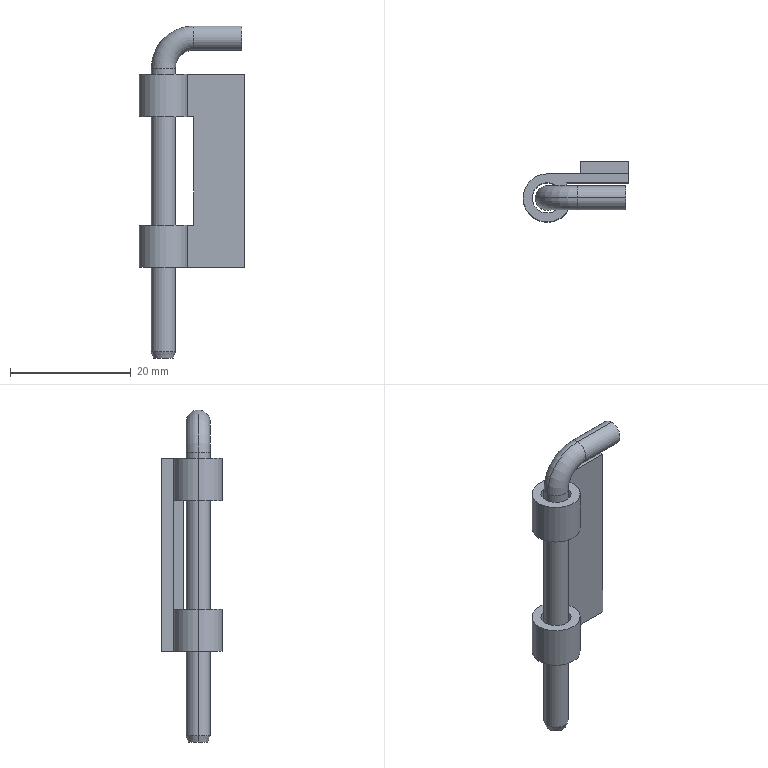Part | STEP file | Latch hinge 001 | 3 solids | 34 faces | box 17.5 x 10 x 55 mm | volume 2208 mm3 | plane 16 | cylinder 14 | torus 2 | cone 2 | commonest cylinder face diameters 8 x6 4 x4 5 x4